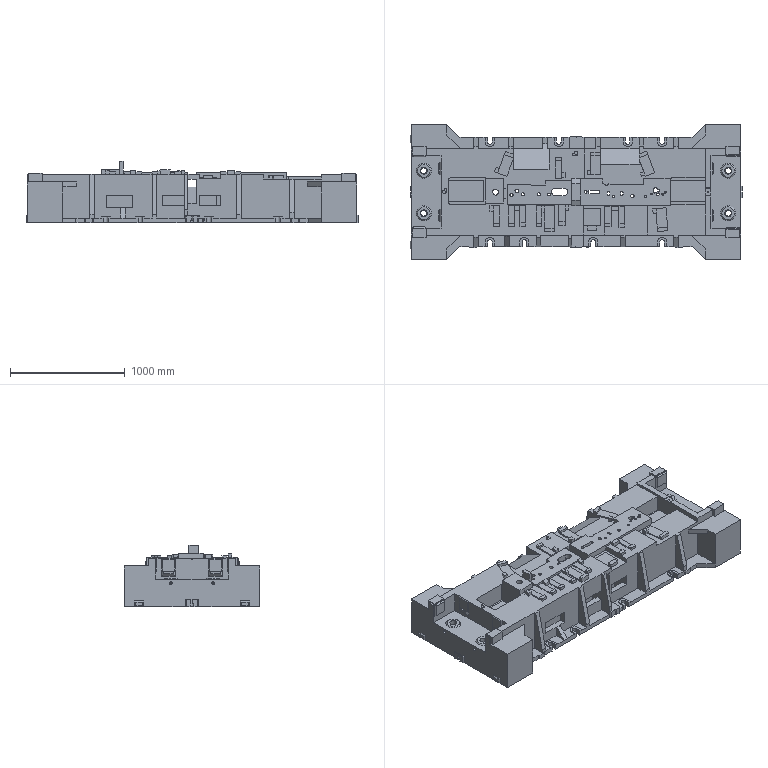Part | NX | features solid 2 | 1 solid | 1012 faces | box 2890 x 1180 x 535 mm | volume 431513223 mm3 | plane 840 | cylinder 139 | spline 26 | cone 7 | commonest cylinder face diameters 20 x46 40 x16 10 x11 80 x8 100 x8 25 x5